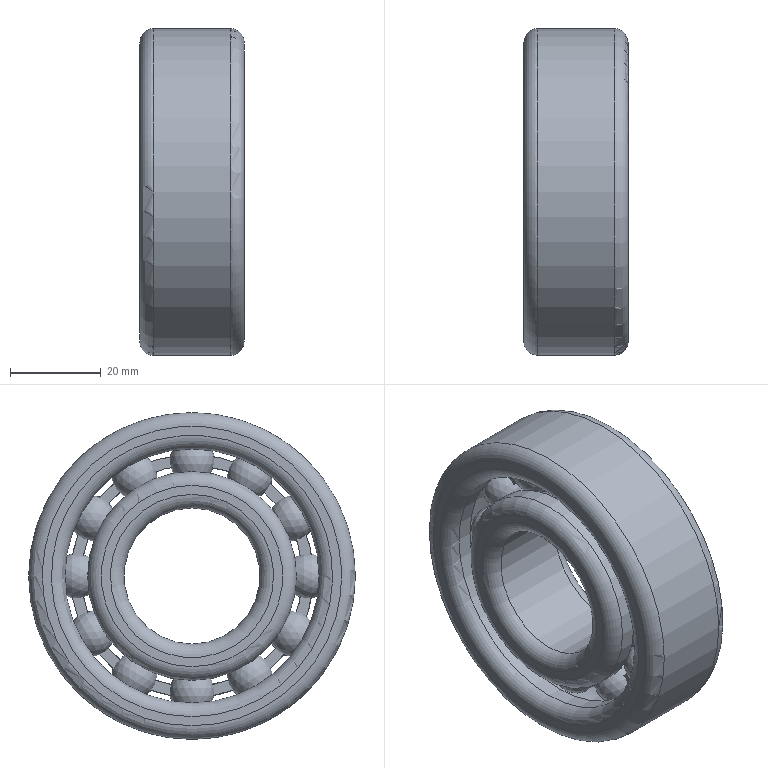Part | NX | features EXTRACT_BODY 12, BLEND 3, DATUM_CSYS 3, SKETCH 2, Container 1, EXTRUDE 1, Geometry Instance 1, Pattern Geometry 1, SHELL 1, SPHERE 1, SUBTRACT 1, SWP104 1 | 16 solids | 40 faces | box 23 x 72 x 72 mm | volume 56238 mm3 | sphere 12 | cylinder 10 | torus 10 | plane 8 | commonest cylinder face diameters 46 x2 48.745 x2 53.552 x2 56 x2 30 x1 72 x1
STEP:
#1=CARTESIAN_POINT('',(0.,26.776,0.));
#2=VERTEX_POINT('',#1);
#3=CARTESIAN_POINT('',(0.,0.,0.));
#4=DIRECTION('',(1.,0.,0.));
#5=DIRECTION('',(0.,1.,0.));
#6=AXIS2_PLACEMENT_3D('',#3,#4,#5);
#7=CIRCLE('',#6,26.776);
#8=EDGE_CURVE('',#2,#2,#7,.F.);
#9=ORIENTED_EDGE('',*,*,#8,.T.);
#10=EDGE_LOOP('',(#9));
#11=FACE_BOUND('',#10,.T.);
#12=CARTESIAN_POINT('',(-1.,0.,-26.776));
#13=VERTEX_POINT('',#12);
#14=CARTESIAN_POINT('',(-1.,0.,0.));
#15=DIRECTION('',(1.,0.,0.));
#16=DIRECTION('',(0.,0.,-1.));
#17=AXIS2_PLACEMENT_3D('',#14,#15,#16);
#18=CIRCLE('',#17,26.776);
#19=EDGE_CURVE('',#13,#13,#18,.F.);
#20=ORIENTED_EDGE('',*,*,#19,.F.);
#21=EDGE_LOOP('',(#20));
#22=FACE_BOUND('',#21,.T.);
#23=CARTESIAN_POINT('',(-7.,0.,0.));
#24=DIRECTION('',(1.,0.,0.));
#25=DIRECTION('',(0.,0.,1.));
#26=AXIS2_PLACEMENT_3D('',#23,#24,#25);
#27=CYLINDRICAL_SURFACE('',#26,26.776);
#28=ADVANCED_FACE('',(#11,#22),#27,.T.);
#29=CARTESIAN_POINT('',(0.,24.373,0.));
#30=VERTEX_POINT('',#29);
#31=CARTESIAN_POINT('',(0.,0.,0.));
#32=DIRECTION('',(1.,0.,0.));
#33=DIRECTION('',(0.,1.,0.));
#34=AXIS2_PLACEMENT_3D('',#31,#32,#33);
#35=CIRCLE('',#34,24.373);
#36=EDGE_CURVE('',#30,#30,#35,.F.);
#37=ORIENTED_EDGE('',*,*,#36,.F.);
#38=EDGE_LOOP('',(#37));
#39=FACE_BOUND('',#38,.T.);
#40=CARTESIAN_POINT('',(-1.,0.,-24.373));
#41=VERTEX_POINT('',#40);
#42=CARTESIAN_POINT('',(-1.,0.,0.));
#43=DIRECTION('',(1.,0.,0.));
#44=DIRECTION('',(0.,0.,-1.));
#45=AXIS2_PLACEMENT_3D('',#42,#43,#44);
#46=CIRCLE('',#45,24.373);
#47=EDGE_CURVE('',#41,#41,#46,.F.);
#48=ORIENTED_EDGE('',*,*,#47,.T.);
#49=EDGE_LOOP('',(#48));
#50=FACE_BOUND('',#49,.T.);
#51=CARTESIAN_POINT('',(-7.,0.,0.));
#52=DIRECTION('',(1.,0.,0.));
#53=DIRECTION('',(0.,0.,1.));
#54=AXIS2_PLACEMENT_3D('',#51,#52,#53);
#55=CYLINDRICAL_SURFACE('',#54,24.373);
#56=ADVANCED_FACE('',(#39,#50),#55,.F.);
#57=ORIENTED_EDGE('',*,*,#8,.F.);
#58=EDGE_LOOP('',(#57));
#59=FACE_BOUND('',#58,.T.);
#60=ORIENTED_EDGE('',*,*,#36,.T.);
#61=EDGE_LOOP('',(#60));
#62=FACE_BOUND('',#61,.T.);
#63=CARTESIAN_POINT('',(0.,0.,0.));
#64=DIRECTION('',(-1.,0.,0.));
#65=DIRECTION('',(0.,0.,-1.));
#66=AXIS2_PLACEMENT_3D('',#63,#64,#65);
#67=PLANE('',#66);
#68=ADVANCED_FACE('',(#59,#62),#67,.F.);
#69=ORIENTED_EDGE('',*,*,#19,.T.);
#70=EDGE_LOOP('',(#69));
#71=FACE_BOUND('',#70,.T.);
#72=ORIENTED_EDGE('',*,*,#47,.F.);
#73=EDGE_LOOP('',(#72));
#74=FACE_BOUND('',#73,.T.);
#75=CARTESIAN_POINT('',(-1.,0.,0.));
#76=DIRECTION('',(-1.,0.,0.));
#77=DIRECTION('',(0.,0.,-1.));
#78=AXIS2_PLACEMENT_3D('',#75,#76,#77);
#79=PLANE('',#78);
#80=ADVANCED_FACE('',(#71,#74),#79,.T.);
#81=CLOSED_SHELL('',(#28,#56,#68,#80));
#82=MANIFOLD_SOLID_BREP('',#81);
#83=CARTESIAN_POINT('',(0.,0.,-20.5));
#84=VERTEX_POINT('',#83);
#85=VERTEX_LOOP('',#84);
#86=FACE_BOUND('',#85,.T.);
#87=CARTESIAN_POINT('',(0.,0.,-25.5));
#88=DIRECTION('',(0.,0.,-1.));
#89=DIRECTION('',(1.,0.,0.));
#90=AXIS2_PLACEMENT_3D('',#87,#88,#89);
#91=SPHERICAL_SURFACE('',#90,5.);
#92=ADVANCED_FACE('',(#86),#91,.T.);
#93=CLOSED_SHELL('',(#92));
#94=MANIFOLD_SOLID_BREP('',#93);
#95=CARTESIAN_POINT('',(0.,-10.25,-17.754));
#96=VERTEX_POINT('',#95);
#97=VERTEX_LOOP('',#96);
#98=FACE_BOUND('',#97,.T.);
#99=CARTESIAN_POINT('',(0.,-12.75,-22.084));
#100=DIRECTION('',(0.,-0.5,-0.866));
#101=DIRECTION('',(1.,0.,0.));
#102=AXIS2_PLACEMENT_3D('',#99,#100,#101);
#103=SPHERICAL_SURFACE('',#102,5.);
#104=ADVANCED_FACE('',(#98),#103,.T.);
#105=CLOSED_SHELL('',(#104));
#106=MANIFOLD_SOLID_BREP('',#105);
#107=CARTESIAN_POINT('',(0.,-17.754,10.25));
#108=VERTEX_POINT('',#107);
#109=VERTEX_LOOP('',#108);
#110=FACE_BOUND('',#109,.T.);
#111=CARTESIAN_POINT('',(0.,-22.084,12.75));
#112=DIRECTION('',(0.,-0.866,0.5));
#113=DIRECTION('',(1.,0.,0.));
#114=AXIS2_PLACEMENT_3D('',#111,#112,#113);
#115=SPHERICAL_SURFACE('',#114,5.);
#116=ADVANCED_FACE('',(#110),#115,.T.);
#117=CLOSED_SHELL('',(#116));
#118=MANIFOLD_SOLID_BREP('',#117);
#119=CARTESIAN_POINT('',(0.,10.25,-17.754));
#120=VERTEX_POINT('',#119);
#121=VERTEX_LOOP('',#120);
#122=FACE_BOUND('',#121,.T.);
#123=CARTESIAN_POINT('',(0.,12.75,-22.084));
#124=DIRECTION('',(0.,0.5,-0.866));
#125=DIRECTION('',(1.,0.,0.));
#126=AXIS2_PLACEMENT_3D('',#123,#124,#125);
#127=SPHERICAL_SURFACE('',#126,5.);
#128=ADVANCED_FACE('',(#122),#127,.T.);
#129=CLOSED_SHELL('',(#128));
#130=MANIFOLD_SOLID_BREP('',#129);
#131=CARTESIAN_POINT('',(0.,-17.754,-10.25));
#132=VERTEX_POINT('',#131);
#133=VERTEX_LOOP('',#132);
#134=FACE_BOUND('',#133,.T.);
#135=CARTESIAN_POINT('',(0.,-22.084,-12.75));
#136=DIRECTION('',(0.,-0.866,-0.5));
#137=DIRECTION('',(1.,0.,0.));
#138=AXIS2_PLACEMENT_3D('',#135,#136,#137);
#139=SPHERICAL_SURFACE('',#138,5.);
#140=ADVANCED_FACE('',(#134),#139,.T.);
#141=CLOSED_SHELL('',(#140));
#142=MANIFOLD_SOLID_BREP('',#141);
#143=CARTESIAN_POINT('',(0.,17.754,-10.25));
#144=VERTEX_POINT('',#143);
#145=VERTEX_LOOP('',#144);
#146=FACE_BOUND('',#145,.T.);
#147=CARTESIAN_POINT('',(0.,22.084,-12.75));
#148=DIRECTION('',(0.,0.866,-0.5));
#149=DIRECTION('',(1.,0.,0.));
#150=AXIS2_PLACEMENT_3D('',#147,#148,#149);
#151=SPHERICAL_SURFACE('',#150,5.);
#152=ADVANCED_FACE('',(#146),#151,.T.);
#153=CLOSED_SHELL('',(#152));
#154=MANIFOLD_SOLID_BREP('',#153);
#155=CARTESIAN_POINT('',(-8.5,0.,-36.));
#156=VERTEX_POINT('',#155);
#157=CARTESIAN_POINT('',(-8.5,0.,0.));
#158=DIRECTION('',(1.,0.,0.));
#159=DIRECTION('',(0.,0.,-1.));
#160=AXIS2_PLACEMENT_3D('',#157,#158,#159);
#161=CIRCLE('',#160,36.);
#162=EDGE_CURVE('',#156,#156,#161,.T.);
#163=ORIENTED_EDGE('',*,*,#162,.T.);
#164=EDGE_LOOP('',(#163));
#165=FACE_BOUND('',#164,.T.);
#166=CARTESIAN_POINT('',(8.5,0.,36.));
#167=VERTEX_POINT('',#166);
#168=CARTESIAN_POINT('',(8.5,0.,0.));
#169=DIRECTION('',(-1.,0.,0.));
#170=DIRECTION('',(0.,0.,1.));
#171=AXIS2_PLACEMENT_3D('',#168,#169,#170);
#172=CIRCLE('',#171,36.);
#173=EDGE_CURVE('',#167,#167,#172,.T.);
#174=ORIENTED_EDGE('',*,*,#173,.T.);
#175=EDGE_LOOP('',(#174));
#176=FACE_BOUND('',#175,.T.);
#177=CARTESIAN_POINT('',(0.,0.,0.));
#178=DIRECTION('',(-1.,0.,0.));
#179=DIRECTION('',(0.,0.,1.));
#180=AXIS2_PLACEMENT_3D('',#177,#178,#179);
#181=CYLINDRICAL_SURFACE('',#180,36.);
#182=ADVANCED_FACE('',(#165,#176),#181,.T.);
#183=CARTESIAN_POINT('',(-11.5,0.,-31.));
#184=VERTEX_POINT('',#183);
#185=CARTESIAN_POINT('',(-11.5,0.,0.));
#186=DIRECTION('',(1.,0.,0.));
#187=DIRECTION('',(0.,0.,-1.));
#188=AXIS2_PLACEMENT_3D('',#185,#186,#187);
#189=CIRCLE('',#188,31.);
#190=EDGE_CURVE('',#184,#184,#189,.T.);
#191=ORIENTED_EDGE('',*,*,#190,.T.);
#192=EDGE_LOOP('',(#191));
#193=FACE_BOUND('',#192,.T.);
#194=CARTESIAN_POINT('',(-11.5,0.,-33.));
#195=VERTEX_POINT('',#194);
#196=CARTESIAN_POINT('',(-11.5,0.,0.));
#197=DIRECTION('',(1.,0.,0.));
#198=DIRECTION('',(0.,0.,-1.));
#199=AXIS2_PLACEMENT_3D('',#196,#197,#198);
#200=CIRCLE('',#199,33.);
#201=EDGE_CURVE('',#195,#195,#200,.F.);
#202=ORIENTED_EDGE('',*,*,#201,.T.);
#203=EDGE_LOOP('',(#202));
#204=FACE_BOUND('',#203,.T.);
#205=CARTESIAN_POINT('',(-11.5,36.,0.));
#206=DIRECTION('',(1.,0.,0.));
#207=DIRECTION('',(0.,0.,-1.));
#208=AXIS2_PLACEMENT_3D('',#205,#206,#207);
#209=PLANE('',#208);
#210=ADVANCED_FACE('',(#193,#204),#209,.F.);
#211=CARTESIAN_POINT('',(-8.5,0.,-28.));
#212=VERTEX_POINT('',#211);
#213=CARTESIAN_POINT('',(-8.5,0.,0.));
#214=DIRECTION('',(1.,0.,0.));
#215=DIRECTION('',(0.,0.,-1.));
#216=AXIS2_PLACEMENT_3D('',#213,#214,#215);
#217=CIRCLE('',#216,28.);
#218=EDGE_CURVE('',#212,#212,#217,.F.);
#219=ORIENTED_EDGE('',*,*,#218,.T.);
#220=EDGE_LOOP('',(#219));
#221=FACE_BOUND('',#220,.T.);
#222=CARTESIAN_POINT('',(-5.062,0.,28.));
#223=VERTEX_POINT('',#222);
#224=CARTESIAN_POINT('',(-5.062,0.,0.));
#225=DIRECTION('',(-1.,0.,0.));
#226=DIRECTION('',(0.,0.,1.));
#227=AXIS2_PLACEMENT_3D('',#224,#225,#226);
#228=CIRCLE('',#227,28.);
#229=EDGE_CURVE('',#223,#223,#228,.T.);
#230=ORIENTED_EDGE('',*,*,#229,.F.);
#231=EDGE_LOOP('',(#230));
#232=FACE_BOUND('',#231,.T.);
#233=CARTESIAN_POINT('',(0.,0.,0.));
#234=DIRECTION('',(-1.,0.,0.));
#235=DIRECTION('',(0.,0.,1.));
#236=AXIS2_PLACEMENT_3D('',#233,#234,#235);
#237=CYLINDRICAL_SURFACE('',#236,28.);
#238=ADVANCED_FACE('',(#221,#232),#237,.F.);
#239=CARTESIAN_POINT('',(5.062,0.,28.));
#240=VERTEX_POINT('',#239);
#241=CARTESIAN_POINT('',(5.062,0.,0.));
#242=DIRECTION('',(-1.,0.,0.));
#243=DIRECTION('',(0.,0.,1.));
#244=AXIS2_PLACEMENT_3D('',#241,#242,#243);
#245=CIRCLE('',#244,28.);
#246=EDGE_CURVE('',#240,#240,#245,.T.);
#247=ORIENTED_EDGE('',*,*,#246,.F.);
#248=EDGE_LOOP('',(#247));
#249=FACE_BOUND('',#248,.T.);
#250=ORIENTED_EDGE('',*,*,#229,.T.);
#251=EDGE_LOOP('',(#250));
#252=FACE_BOUND('',#251,.T.);
#253=CARTESIAN_POINT('',(0.,0.,0.));
#254=DIRECTION('',(-1.,0.,0.));
#255=DIRECTION('',(0.,0.,1.));
#256=AXIS2_PLACEMENT_3D('',#253,#254,#255);
#257=TOROIDAL_SURFACE('',#256,25.5,5.646);
#258=ADVANCED_FACE('',(#249,#252),#257,.F.);
#259=CARTESIAN_POINT('',(8.5,0.,28.));
#260=VERTEX_POINT('',#259);
#261=CARTESIAN_POINT('',(8.5,0.,0.));
#262=DIRECTION('',(-1.,0.,0.));
#263=DIRECTION('',(0.,0.,1.));
#264=AXIS2_PLACEMENT_3D('',#261,#262,#263);
#265=CIRCLE('',#264,28.);
#266=EDGE_CURVE('',#260,#260,#265,.F.);
#267=ORIENTED_EDGE('',*,*,#266,.T.);
#268=EDGE_LOOP('',(#267));
#269=FACE_BOUND('',#268,.T.);
#270=ORIENTED_EDGE('',*,*,#246,.T.);
#271=EDGE_LOOP('',(#270));
#272=FACE_BOUND('',#271,.T.);
#273=CARTESIAN_POINT('',(0.,0.,0.));
#274=DIRECTION('',(-1.,0.,0.));
#275=DIRECTION('',(0.,0.,1.));
#276=AXIS2_PLACEMENT_3D('',#273,#274,#275);
#277=CYLINDRICAL_SURFACE('',#276,28.);
#278=ADVANCED_FACE('',(#269,#272),#277,.F.);
#279=CARTESIAN_POINT('',(11.5,0.,31.));
#280=VERTEX_POINT('',#279);
#281=CARTESIAN_POINT('',(11.5,0.,0.));
#282=DIRECTION('',(-1.,0.,0.));
#283=DIRECTION('',(0.,0.,1.));
#284=AXIS2_PLACEMENT_3D('',#281,#282,#283);
#285=CIRCLE('',#284,31.);
#286=EDGE_CURVE('',#280,#280,#285,.T.);
#287=ORIENTED_EDGE('',*,*,#286,.T.);
#288=EDGE_LOOP('',(#287));
#289=FACE_BOUND('',#288,.T.);
#290=CARTESIAN_POINT('',(11.5,0.,33.));
#291=VERTEX_POINT('',#290);
#292=CARTESIAN_POINT('',(11.5,0.,0.));
#293=DIRECTION('',(-1.,0.,0.));
#294=DIRECTION('',(0.,0.,1.));
#295=AXIS2_PLACEMENT_3D('',#292,#293,#294);
#296=CIRCLE('',#295,33.);
#297=EDGE_CURVE('',#291,#291,#296,.F.);
#298=ORIENTED_EDGE('',*,*,#297,.T.);
#299=EDGE_LOOP('',(#298));
#300=FACE_BOUND('',#299,.T.);
#301=CARTESIAN_POINT('',(11.5,28.,0.));
#302=DIRECTION('',(-1.,0.,0.));
#303=DIRECTION('',(0.,0.,1.));
#304=AXIS2_PLACEMENT_3D('',#301,#302,#303);
#305=PLANE('',#304);
#306=ADVANCED_FACE('',(#289,#300),#305,.F.);
#307=ORIENTED_EDGE('',*,*,#190,.F.);
#308=EDGE_LOOP('',(#307));
#309=FACE_BOUND('',#308,.T.);
#310=ORIENTED_EDGE('',*,*,#218,.F.);
#311=EDGE_LOOP('',(#310));
#312=FACE_BOUND('',#311,.T.);
#313=CARTESIAN_POINT('',(-8.5,0.,0.));
#314=DIRECTION('',(1.,0.,0.));
#315=DIRECTION('',(0.,0.,-1.));
#316=AXIS2_PLACEMENT_3D('',#313,#314,#315);
#317=TOROIDAL_SURFACE('',#316,31.,3.);
#318=ADVANCED_FACE('',(#309,#312),#317,.T.);
#319=ORIENTED_EDGE('',*,*,#266,.F.);
#320=EDGE_LOOP('',(#319));
#321=FACE_BOUND('',#320,.T.);
#322=ORIENTED_EDGE('',*,*,#286,.F.);
#323=EDGE_LOOP('',(#322));
#324=FACE_BOUND('',#323,.T.);
#325=CARTESIAN_POINT('',(8.5,0.,0.));
#326=DIRECTION('',(-1.,0.,0.));
#327=DIRECTION('',(0.,0.,1.));
#328=AXIS2_PLACEMENT_3D('',#325,#326,#327);
#329=TOROIDAL_SURFACE('',#328,31.,3.);
#330=ADVANCED_FACE('',(#321,#324),#329,.T.);
#331=ORIENTED_EDGE('',*,*,#162,.F.);
#332=EDGE_LOOP('',(#331));
#333=FACE_BOUND('',#332,.T.);
#334=ORIENTED_EDGE('',*,*,#201,.F.);
#335=EDGE_LOOP('',(#334));
#336=FACE_BOUND('',#335,.T.);
#337=CARTESIAN_POINT('',(-8.5,0.,0.));
#338=DIRECTION('',(1.,0.,0.));
#339=DIRECTION('',(0.,0.,-1.));
#340=AXIS2_PLACEMENT_3D('',#337,#338,#339);
#341=TOROIDAL_SURFACE('',#340,33.,3.);
#342=ADVANCED_FACE('',(#333,#336),#341,.T.);
#343=ORIENTED_EDGE('',*,*,#297,.F.);
#344=EDGE_LOOP('',(#343));
#345=FACE_BOUND('',#344,.T.);
#346=ORIENTED_EDGE('',*,*,#173,.F.);
#347=EDGE_LOOP('',(#346));
#348=FACE_BOUND('',#347,.T.);
#349=CARTESIAN_POINT('',(8.5,0.,0.));
#350=DIRECTION('',(-1.,0.,0.));
#351=DIRECTION('',(0.,0.,1.));
#352=AXIS2_PLACEMENT_3D('',#349,#350,#351);
#353=TOROIDAL_SURFACE('',#352,33.,3.);
#354=ADVANCED_FACE('',(#345,#348),#353,.T.);
#355=CLOSED_SHELL('',(#182,#210,#238,#258,#278,#306,#318,#330,#342,#354));
#356=MANIFOLD_SOLID_BREP('',#355);
#357=CARTESIAN_POINT('',(0.,-10.25,17.754));
#358=VERTEX_POINT('',#357);
#359=VERTEX_LOOP('',#358);
#360=FACE_BOUND('',#359,.T.);
#361=CARTESIAN_POINT('',(0.,-12.75,22.084));
#362=DIRECTION('',(0.,-0.5,0.866));
#363=DIRECTION('',(1.,0.,0.));
#364=AXIS2_PLACEMENT_3D('',#361,#362,#363);
#365=SPHERICAL_SURFACE('',#364,5.);
#366=ADVANCED_FACE('',(#360),#365,.T.);
#367=CLOSED_SHELL('',(#366));
#368=MANIFOLD_SOLID_BREP('',#367);
#369=CARTESIAN_POINT('',(0.,17.754,10.25));
#370=VERTEX_POINT('',#369);
#371=VERTEX_LOOP('',#370);
#372=FACE_BOUND('',#371,.T.);
#373=CARTESIAN_POINT('',(0.,22.084,12.75));
#374=DIRECTION('',(0.,0.866,0.5));
#375=DIRECTION('',(1.,0.,0.));
#376=AXIS2_PLACEMENT_3D('',#373,#374,#375);
#377=SPHERICAL_SURFACE('',#376,5.);
#378=ADVANCED_FACE('',(#372),#377,.T.);
#379=CLOSED_SHELL('',(#378));
#380=MANIFOLD_SOLID_BREP('',#379);
#381=CARTESIAN_POINT('',(0.,10.25,17.754));
#382=VERTEX_POINT('',#381);
#383=VERTEX_LOOP('',#382);
#384=FACE_BOUND('',#383,.T.);
#385=CARTESIAN_POINT('',(0.,12.75,22.084));
#386=DIRECTION('',(0.,0.5,0.866));
#387=DIRECTION('',(1.,0.,0.));
#388=AXIS2_PLACEMENT_3D('',#385,#386,#387);
#389=SPHERICAL_SURFACE('',#388,5.);
#390=ADVANCED_FACE('',(#384),#389,.T.);
#391=CLOSED_SHELL('',(#390));
#392=MANIFOLD_SOLID_BREP('',#391);
#393=CARTESIAN_POINT('',(-8.5,0.,23.));
#394=VERTEX_POINT('',#393);
#395=CARTESIAN_POINT('',(-8.5,0.,0.));
#396=DIRECTION('',(-1.,0.,0.));
#397=DIRECTION('',(0.,0.,1.));
#398=AXIS2_PLACEMENT_3D('',#395,#396,#397);
#399=CIRCLE('',#398,23.);
#400=EDGE_CURVE('',#394,#394,#399,.F.);
#401=ORIENTED_EDGE('',*,*,#400,.T.);
#402=EDGE_LOOP('',(#401));
#403=FACE_BOUND('',#402,.T.);
#404=CARTESIAN_POINT('',(-5.062,0.,23.));
#405=VERTEX_POINT('',#404);
#406=CARTESIAN_POINT('',(-5.062,0.,0.));
#407=DIRECTION('',(-1.,0.,0.));
#408=DIRECTION('',(0.,0.,1.));
#409=AXIS2_PLACEMENT_3D('',#406,#407,#408);
#410=CIRCLE('',#409,23.);
#411=EDGE_CURVE('',#405,#405,#410,.T.);
#412=ORIENTED_EDGE('',*,*,#411,.T.);
#413=EDGE_LOOP('',(#412));
#414=FACE_BOUND('',#413,.T.);
#415=CARTESIAN_POINT('',(0.,0.,0.));
#416=DIRECTION('',(-1.,0.,0.));
#417=DIRECTION('',(0.,0.,1.));
#418=AXIS2_PLACEMENT_3D('',#415,#416,#417);
#419=CYLINDRICAL_SURFACE('',#418,23.);
#420=ADVANCED_FACE('',(#403,#414),#419,.T.);
#421=CARTESIAN_POINT('',(5.062,0.,23.));
#422=VERTEX_POINT('',#421);
#423=CARTESIAN_POINT('',(5.062,0.,0.));
#424=DIRECTION('',(-1.,0.,0.));
#425=DIRECTION('',(0.,0.,1.));
#426=AXIS2_PLACEMENT_3D('',#423,#424,#425);
#427=CIRCLE('',#426,23.);
#428=EDGE_CURVE('',#422,#422,#427,.T.);
#429=ORIENTED_EDGE('',*,*,#428,.T.);
#430=EDGE_LOOP('',(#429));
#431=FACE_BOUND('',#430,.T.);
#432=ORIENTED_EDGE('',*,*,#411,.F.);
#433=EDGE_LOOP('',(#432));
#434=FACE_BOUND('',#433,.T.);
#435=CARTESIAN_POINT('',(0.,0.,0.));
#436=DIRECTION('',(-1.,0.,0.));
#437=DIRECTION('',(0.,0.,1.));
#438=AXIS2_PLACEMENT_3D('',#435,#436,#437);
#439=TOROIDAL_SURFACE('',#438,25.5,5.646);
#440=ADVANCED_FACE('',(#431,#434),#439,.F.);
#441=CARTESIAN_POINT('',(8.5,0.,-23.));
#442=VERTEX_POINT('',#441);
#443=CARTESIAN_POINT('',(8.5,0.,0.));
#444=DIRECTION('',(1.,0.,0.));
#445=DIRECTION('',(0.,0.,-1.));
#446=AXIS2_PLACEMENT_3D('',#443,#444,#445);
#447=CIRCLE('',#446,23.);
#448=EDGE_CURVE('',#442,#442,#447,.F.);
#449=ORIENTED_EDGE('',*,*,#448,.T.);
#450=EDGE_LOOP('',(#449));
#451=FACE_BOUND('',#450,.T.);
#452=ORIENTED_EDGE('',*,*,#428,.F.);
#453=EDGE_LOOP('',(#452));
#454=FACE_BOUND('',#453,.T.);
#455=CARTESIAN_POINT('',(0.,0.,0.));
#456=DIRECTION('',(-1.,0.,0.));
#457=DIRECTION('',(0.,0.,1.));
#458=AXIS2_PLACEMENT_3D('',#455,#456,#457);
#459=CYLINDRICAL_SURFACE('',#458,23.);
#460=ADVANCED_FACE('',(#451,#454),#459,.T.);
#461=CARTESIAN_POINT('',(11.5,0.,-18.));
#462=VERTEX_POINT('',#461);
#463=CARTESIAN_POINT('',(11.5,0.,0.));
#464=DIRECTION('',(1.,0.,0.));
#465=DIRECTION('',(0.,0.,-1.));
#466=AXIS2_PLACEMENT_3D('',#463,#464,#465);
#467=CIRCLE('',#466,18.);
#468=EDGE_CURVE('',#462,#462,#467,.F.);
#469=ORIENTED_EDGE('',*,*,#468,.T.);
#470=EDGE_LOOP('',(#469));
#471=FACE_BOUND('',#470,.T.);
#472=CARTESIAN_POINT('',(11.5,0.,-20.));
#473=VERTEX_POINT('',#472);
#474=CARTESIAN_POINT('',(11.5,0.,0.));
#475=DIRECTION('',(1.,0.,0.));
#476=DIRECTION('',(0.,0.,-1.));
#477=AXIS2_PLACEMENT_3D('',#474,#475,#476);
#478=CIRCLE('',#477,20.);
#479=EDGE_CURVE('',#473,#473,#478,.T.);
#480=ORIENTED_EDGE('',*,*,#479,.T.);
#481=EDGE_LOOP('',(#480));
#482=FACE_BOUND('',#481,.T.);
#483=CARTESIAN_POINT('',(11.5,23.,0.));
#484=DIRECTION('',(1.,0.,0.));
#485=DIRECTION('',(0.,0.,-1.));
#486=AXIS2_PLACEMENT_3D('',#483,#484,#485);
#487=PLANE('',#486);
#488=ADVANCED_FACE('',(#471,#482),#487,.T.);
#489=CARTESIAN_POINT('',(-8.5,0.,15.));
#490=VERTEX_POINT('',#489);
#491=CARTESIAN_POINT('',(-8.5,0.,0.));
#492=DIRECTION('',(-1.,0.,0.));
#493=DIRECTION('',(0.,0.,1.));
#494=AXIS2_PLACEMENT_3D('',#491,#492,#493);
#495=CIRCLE('',#494,15.);
#496=EDGE_CURVE('',#490,#490,#495,.T.);
#497=ORIENTED_EDGE('',*,*,#496,.T.);
#498=EDGE_LOOP('',(#497));
#499=FACE_BOUND('',#498,.T.);
#500=CARTESIAN_POINT('',(8.5,0.,-15.));
#501=VERTEX_POINT('',#500);
#502=CARTESIAN_POINT('',(8.5,0.,0.));
#503=DIRECTION('',(1.,0.,0.));
#504=DIRECTION('',(0.,0.,-1.));
#505=AXIS2_PLACEMENT_3D('',#502,#503,#504);
#506=CIRCLE('',#505,15.);
#507=EDGE_CURVE('',#501,#501,#506,.T.);
#508=ORIENTED_EDGE('',*,*,#507,.T.);
#509=EDGE_LOOP('',(#508));
#510=FACE_BOUND('',#509,.T.);
#511=CARTESIAN_POINT('',(0.,0.,0.));
#512=DIRECTION('',(-1.,0.,0.));
#513=DIRECTION('',(0.,0.,1.));
#514=AXIS2_PLACEMENT_3D('',#511,#512,#513);
#515=CYLINDRICAL_SURFACE('',#514,15.);
#516=ADVANCED_FACE('',(#499,#510),#515,.F.);
#517=CARTESIAN_POINT('',(-11.5,0.,18.));
#518=VERTEX_POINT('',#517);
#519=CARTESIAN_POINT('',(-11.5,0.,0.));
#520=DIRECTION('',(-1.,0.,0.));
#521=DIRECTION('',(0.,0.,1.));
#522=AXIS2_PLACEMENT_3D('',#519,#520,#521);
#523=CIRCLE('',#522,18.);
#524=EDGE_CURVE('',#518,#518,#523,.F.);
#525=ORIENTED_EDGE('',*,*,#524,.T.);
#526=EDGE_LOOP('',(#525));
#527=FACE_BOUND('',#526,.T.);
#528=CARTESIAN_POINT('',(-11.5,0.,20.));
#529=VERTEX_POINT('',#528);
#530=CARTESIAN_POINT('',(-11.5,0.,0.));
#531=DIRECTION('',(-1.,0.,0.));
#532=DIRECTION('',(0.,0.,1.));
#533=AXIS2_PLACEMENT_3D('',#530,#531,#532);
#534=CIRCLE('',#533,20.);
#535=EDGE_CURVE('',#529,#529,#534,.T.);
#536=ORIENTED_EDGE('',*,*,#535,.T.);
#537=EDGE_LOOP('',(#536));
#538=FACE_BOUND('',#537,.T.);
#539=CARTESIAN_POINT('',(-11.5,15.,0.));
#540=DIRECTION('',(-1.,0.,0.));
#541=DIRECTION('',(0.,0.,1.));
#542=AXIS2_PLACEMENT_3D('',#539,#540,#541);
#543=PLANE('',#542);
#544=ADVANCED_FACE('',(#527,#538),#543,.T.);
#545=ORIENTED_EDGE('',*,*,#400,.F.);
#546=EDGE_LOOP('',(#545));
#547=FACE_BOUND('',#546,.T.);
#548=ORIENTED_EDGE('',*,*,#535,.F.);
#549=EDGE_LOOP('',(#548));
#550=FACE_BOUND('',#549,.T.);
#551=CARTESIAN_POINT('',(-8.5,0.,0.));
#552=DIRECTION('',(-1.,0.,0.));
#553=DIRECTION('',(0.,0.,1.));
#554=AXIS2_PLACEMENT_3D('',#551,#552,#553);
#555=TOROIDAL_SURFACE('',#554,20.,3.);
#556=ADVANCED_FACE('',(#547,#550),#555,.T.);
#557=ORIENTED_EDGE('',*,*,#479,.F.);
#558=EDGE_LOOP('',(#557));
#559=FACE_BOUND('',#558,.T.);
#560=ORIENTED_EDGE('',*,*,#448,.F.);
#561=EDGE_LOOP('',(#560));
#562=FACE_BOUND('',#561,.T.);
#563=CARTESIAN_POINT('',(8.5,0.,0.));
#564=DIRECTION('',(1.,0.,0.));
#565=DIRECTION('',(0.,0.,-1.));
#566=AXIS2_PLACEMENT_3D('',#563,#564,#565);
#567=TOROIDAL_SURFACE('',#566,20.,3.);
#568=ADVANCED_FACE('',(#559,#562),#567,.T.);
#569=ORIENTED_EDGE('',*,*,#524,.F.);
#570=EDGE_LOOP('',(#569));
#571=FACE_BOUND('',#570,.T.);
#572=ORIENTED_EDGE('',*,*,#496,.F.);
#573=EDGE_LOOP('',(#572));
#574=FACE_BOUND('',#573,.T.);
#575=CARTESIAN_POINT('',(-8.5,0.,0.));
#576=DIRECTION('',(-1.,0.,0.));
#577=DIRECTION('',(0.,0.,1.));
#578=AXIS2_PLACEMENT_3D('',#575,#576,#577);
#579=TOROIDAL_SURFACE('',#578,18.,3.);
#580=ADVANCED_FACE('',(#571,#574),#579,.T.);
#581=ORIENTED_EDGE('',*,*,#507,.F.);
#582=EDGE_LOOP('',(#581));
#583=FACE_BOUND('',#582,.T.);
#584=ORIENTED_EDGE('',*,*,#468,.F.);
#585=EDGE_LOOP('',(#584));
#586=FACE_BOUND('',#585,.T.);
#587=CARTESIAN_POINT('',(8.5,0.,0.));
#588=DIRECTION('',(1.,0.,0.));
#589=DIRECTION('',(0.,0.,-1.));
#590=AXIS2_PLACEMENT_3D('',#587,#588,#589);
#591=TOROIDAL_SURFACE('',#590,18.,3.);
#592=ADVANCED_FACE('',(#583,#586),#591,.T.);
#593=CLOSED_SHELL('',(#420,#440,#460,#488,#516,#544,#556,#568,#580,#592));
#594=MANIFOLD_SOLID_BREP('',#593);
#595=CARTESIAN_POINT('',(0.,26.776,0.));
#596=VERTEX_POINT('',#595);
#597=CARTESIAN_POINT('',(0.,0.,0.));
#598=DIRECTION('',(1.,0.,0.));
#599=DIRECTION('',(0.,1.,0.));
#600=AXIS2_PLACEMENT_3D('',#597,#598,#599);
#601=CIRCLE('',#600,26.776);
#602=EDGE_CURVE('',#596,#596,#601,.T.);
#603=ORIENTED_EDGE('',*,*,#602,.T.);
#604=EDGE_LOOP('',(#603));
#605=FACE_BOUND('',#604,.T.);
#606=CARTESIAN_POINT('',(1.,0.,-26.776));
#607=VERTEX_POINT('',#606);
#608=CARTESIAN_POINT('',(1.,0.,0.));
#609=DIRECTION('',(1.,0.,0.));
#610=DIRECTION('',(0.,0.,-1.));
#611=AXIS2_PLACEMENT_3D('',#608,#609,#610);
#612=CIRCLE('',#611,26.776);
#613=EDGE_CURVE('',#607,#607,#612,.T.);
#614=ORIENTED_EDGE('',*,*,#613,.F.);
#615=EDGE_LOOP('',(#614));
#616=FACE_BOUND('',#615,.T.);
#617=CARTESIAN_POINT('',(7.,0.,0.));
#618=DIRECTION('',(-1.,0.,0.));
#619=DIRECTION('',(0.,0.,1.));
#620=AXIS2_PLACEMENT_3D('',#617,#618,#619);
#621=CYLINDRICAL_SURFACE('',#620,26.776);
#622=ADVANCED_FACE('',(#605,#616),#621,.T.);
#623=CARTESIAN_POINT('',(0.,24.373,0.));
#624=VERTEX_POINT('',#623);
#625=CARTESIAN_POINT('',(0.,0.,0.));
#626=DIRECTION('',(1.,0.,0.));
#627=DIRECTION('',(0.,1.,0.));
#628=AXIS2_PLACEMENT_3D('',#625,#626,#627);
#629=CIRCLE('',#628,24.373);
#630=EDGE_CURVE('',#624,#624,#629,.T.);
#631=ORIENTED_EDGE('',*,*,#630,.F.);
#632=EDGE_LOOP('',(#631));
#633=FACE_BOUND('',#632,.T.);
#634=CARTESIAN_POINT('',(1.,0.,-24.373));
#635=VERTEX_POINT('',#634);
#636=CARTESIAN_POINT('',(1.,0.,0.));
#637=DIRECTION('',(1.,0.,0.));
#638=DIRECTION('',(0.,0.,-1.));
#639=AXIS2_PLACEMENT_3D('',#636,#637,#638);
#640=CIRCLE('',#639,24.373);
#641=EDGE_CURVE('',#635,#635,#640,.T.);
#642=ORIENTED_EDGE('',*,*,#641,.T.);
#643=EDGE_LOOP('',(#642));
#644=FACE_BOUND('',#643,.T.);
#645=CARTESIAN_POINT('',(7.,0.,0.));
#646=DIRECTION('',(-1.,0.,0.));
#647=DIRECTION('',(0.,0.,1.));
#648=AXIS2_PLACEMENT_3D('',#645,#646,#647);
#649=CYLINDRICAL_SURFACE('',#648,24.373);
#650=ADVANCED_FACE('',(#633,#644),#649,.F.);
#651=ORIENTED_EDGE('',*,*,#602,.F.);
#652=EDGE_LOOP('',(#651));
#653=FACE_BOUND('',#652,.T.);
#654=ORIENTED_EDGE('',*,*,#630,.T.);
#655=EDGE_LOOP('',(#654));
#656=FACE_BOUND('',#655,.T.);
#657=CARTESIAN_POINT('',(0.,0.,0.));
#658=DIRECTION('',(1.,0.,0.));
#659=DIRECTION('',(0.,0.,-1.));
#660=AXIS2_PLACEMENT_3D('',#657,#658,#659);
#661=PLANE('',#660);
#662=ADVANCED_FACE('',(#653,#656),#661,.F.);
#663=ORIENTED_EDGE('',*,*,#613,.T.);
#664=EDGE_LOOP('',(#663));
#665=FACE_BOUND('',#664,.T.);
#666=ORIENTED_EDGE('',*,*,#641,.F.);
#667=EDGE_LOOP('',(#666));
#668=FACE_BOUND('',#667,.T.);
#669=CARTESIAN_POINT('',(1.,0.,0.));
#670=DIRECTION('',(1.,0.,0.));
#671=DIRECTION('',(0.,0.,-1.));
#672=AXIS2_PLACEMENT_3D('',#669,#670,#671);
#673=PLANE('',#672);
#674=ADVANCED_FACE('',(#665,#668),#673,.T.);
#675=CLOSED_SHELL('',(#622,#650,#662,#674));
#676=MANIFOLD_SOLID_BREP('',#675);
#677=CARTESIAN_POINT('',(0.,-20.5,0.));
#678=VERTEX_POINT('',#677);
#679=VERTEX_LOOP('',#678);
#680=FACE_BOUND('',#679,.T.);
#681=CARTESIAN_POINT('',(0.,-25.5,0.));
#682=DIRECTION('',(0.,-1.,0.));
#683=DIRECTION('',(1.,0.,0.));
#684=AXIS2_PLACEMENT_3D('',#681,#682,#683);
#685=SPHERICAL_SURFACE('',#684,5.);
#686=ADVANCED_FACE('',(#680),#685,.T.);
#687=CLOSED_SHELL('',(#686));
#688=MANIFOLD_SOLID_BREP('',#687);
#689=CARTESIAN_POINT('',(0.,20.5,0.));
#690=VERTEX_POINT('',#689);
#691=VERTEX_LOOP('',#690);
#692=FACE_BOUND('',#691,.T.);
#693=CARTESIAN_POINT('',(0.,25.5,0.));
#694=DIRECTION('',(0.,1.,0.));
#695=DIRECTION('',(1.,0.,0.));
#696=AXIS2_PLACEMENT_3D('',#693,#694,#695);
#697=SPHERICAL_SURFACE('',#696,5.);
#698=ADVANCED_FACE('',(#692),#697,.T.);
#699=CLOSED_SHELL('',(#698));
#700=MANIFOLD_SOLID_BREP('',#699);
#701=CARTESIAN_POINT('',(0.,0.,20.5));
#702=VERTEX_POINT('',#701);
#703=VERTEX_LOOP('',#702);
#704=FACE_BOUND('',#703,.T.);
#705=CARTESIAN_POINT('',(0.,0.,25.5));
#706=DIRECTION('',(0.,0.,1.));
#707=DIRECTION('',(1.,0.,0.));
#708=AXIS2_PLACEMENT_3D('',#705,#706,#707);
#709=SPHERICAL_SURFACE('',#708,5.);
#710=ADVANCED_FACE('',(#704),#709,.T.);
#711=CLOSED_SHELL('',(#710));
#712=MANIFOLD_SOLID_BREP('',#711);
#713=(LENGTH_UNIT()NAMED_UNIT(*)SI_UNIT(.MILLI.,.METRE.));
#714=UNCERTAINTY_MEASURE_WITH_UNIT(LENGTH_MEASURE(0.00001),#713,'','');
#715=(NAMED_UNIT(*)PLANE_ANGLE_UNIT()SI_UNIT($,.RADIAN.));
#716=(NAMED_UNIT(*)SI_UNIT($,.STERADIAN.)SOLID_ANGLE_UNIT());
#717=(GEOMETRIC_REPRESENTATION_CONTEXT(3)GLOBAL_UNCERTAINTY_ASSIGNED_CONTEXT((#714))GLOBAL_UNIT_ASSIGNED_CONTEXT((#713,#715,#716))REPRESENTATION_CONTEXT('',''));
#718=ADVANCED_BREP_SHAPE_REPRESENTATION('',(#82,#94,#106,#118,#130,#142,#154,#356,#368,#380,#392,#594,#676,#688,#700,#712),#717);